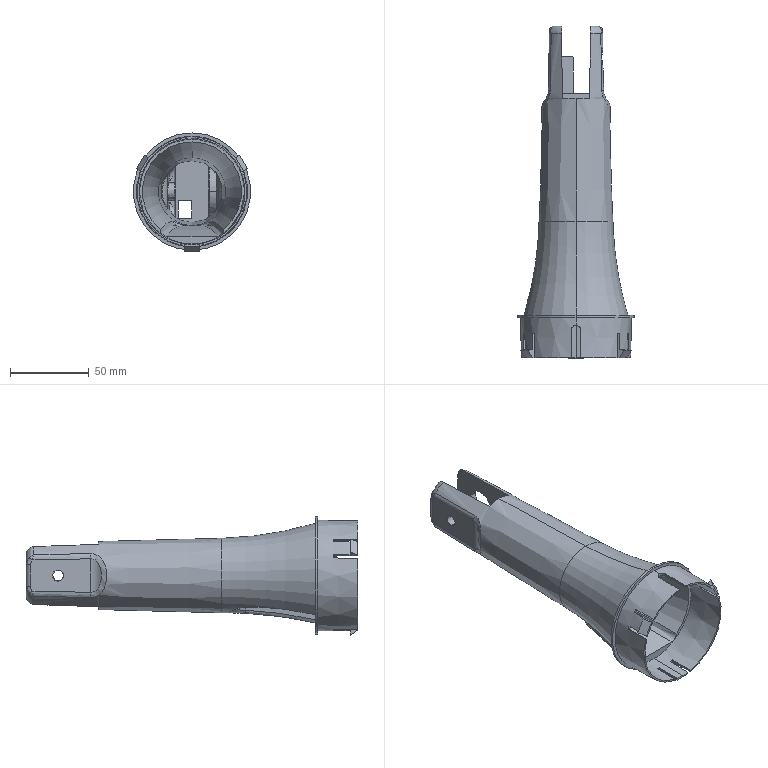Part | STEP file | Torre - produto - 1 cav | 1 solid | 167 faces | box 74.278 x 210.114 x 74.851 mm | volume 69097 mm3 | plane 80 | spline 34 | cone 22 | cylinder 16 | torus 13 | sphere 2 | commonest cylinder face diameters 1.018 x2 2.035 x2 6.105 x2 20.711 x2 24.781 x2 28.622 x2